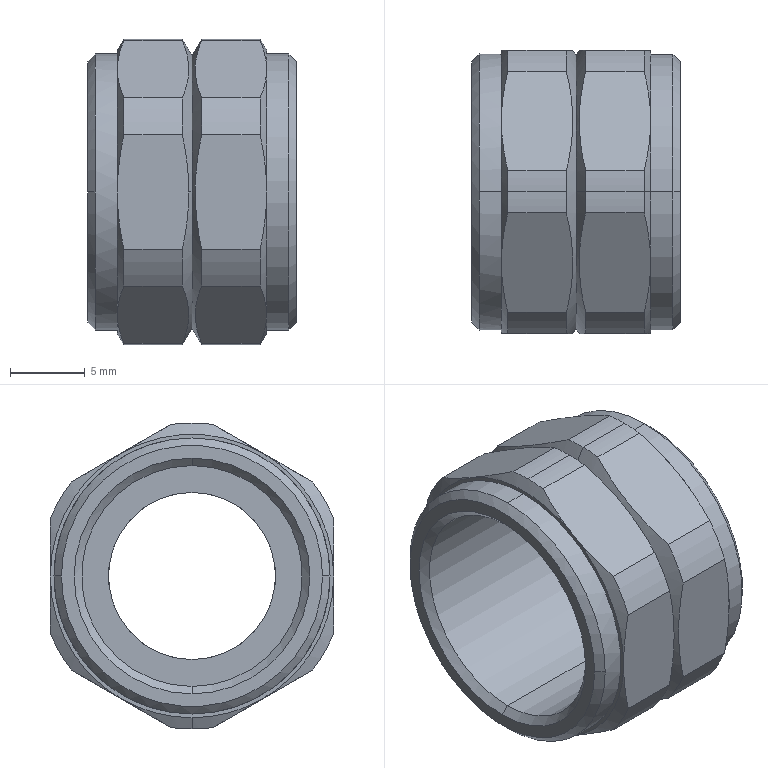Part | STEP file | 8C | 1 solid | 65 faces | box 14 x 19 x 20.5 mm | volume 1899 mm3 | cone 26 | cylinder 22 | plane 17 | commonest cylinder face diameters 20.5 x14 18.5 x4 11.2 x2 14.8 x2